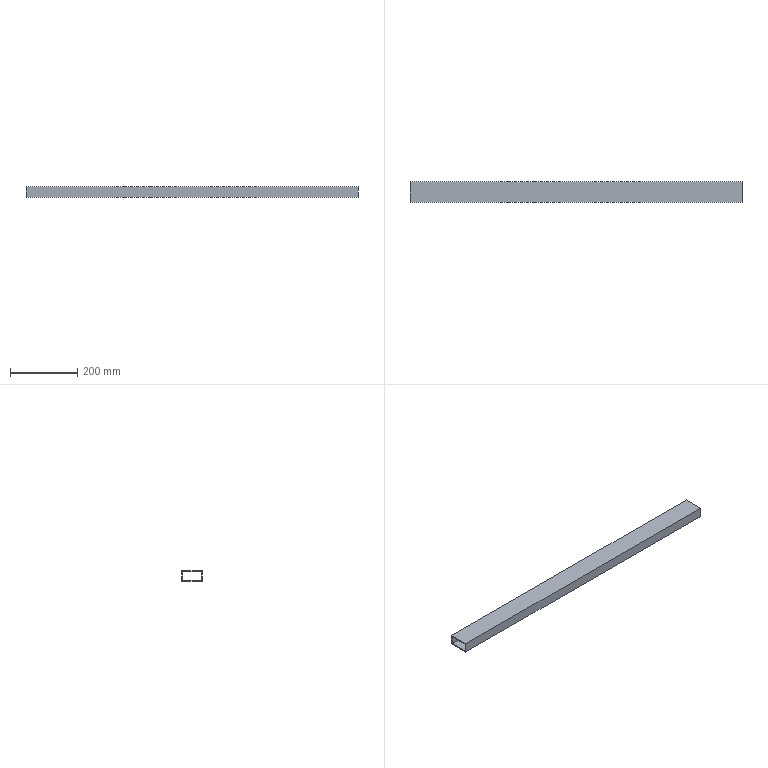Part | SolidWorks | features Cut 1, Extrusion 1 | 1 solid | 10 faces | box 986 x 60 x 30 mm | volume 496944 mm3 | plane 10
STEP:
#1=CARTESIAN_POINT('',(493.,-27.,27.));
#2=VERTEX_POINT('',#1);
#3=CARTESIAN_POINT('',(493.,27.,27.));
#4=VERTEX_POINT('',#3);
#5=CARTESIAN_POINT('',(493.,30.,27.));
#6=DIRECTION('',(0.,1.,0.));
#7=VECTOR('',#6,1000.);
#8=LINE('',#5,#7);
#9=EDGE_CURVE('',#2,#4,#8,.T.);
#10=ORIENTED_EDGE('',*,*,#9,.T.);
#11=CARTESIAN_POINT('',(493.,27.,3.));
#12=VERTEX_POINT('',#11);
#13=CARTESIAN_POINT('',(493.,27.,30.));
#14=DIRECTION('',(0.,0.,-1.));
#15=VECTOR('',#14,1000.);
#16=LINE('',#13,#15);
#17=EDGE_CURVE('',#4,#12,#16,.T.);
#18=ORIENTED_EDGE('',*,*,#17,.T.);
#19=CARTESIAN_POINT('',(493.,-27.,3.));
#20=VERTEX_POINT('',#19);
#21=CARTESIAN_POINT('',(493.,30.,3.));
#22=DIRECTION('',(0.,-1.,0.));
#23=VECTOR('',#22,1000.);
#24=LINE('',#21,#23);
#25=EDGE_CURVE('',#12,#20,#24,.T.);
#26=ORIENTED_EDGE('',*,*,#25,.T.);
#27=CARTESIAN_POINT('',(493.,-27.,30.));
#28=DIRECTION('',(0.,0.,1.));
#29=VECTOR('',#28,1000.);
#30=LINE('',#27,#29);
#31=EDGE_CURVE('',#20,#2,#30,.T.);
#32=ORIENTED_EDGE('',*,*,#31,.T.);
#33=EDGE_LOOP('',(#10,#18,#26,#32));
#34=FACE_BOUND('',#33,.T.);
#35=CARTESIAN_POINT('',(493.,-30.,0.));
#36=VERTEX_POINT('',#35);
#37=CARTESIAN_POINT('',(493.,30.,0.));
#38=VERTEX_POINT('',#37);
#39=CARTESIAN_POINT('',(493.,30.,0.));
#40=DIRECTION('',(0.,1.,0.));
#41=VECTOR('',#40,1000.);
#42=LINE('',#39,#41);
#43=EDGE_CURVE('',#36,#38,#42,.T.);
#44=ORIENTED_EDGE('',*,*,#43,.T.);
#45=CARTESIAN_POINT('',(493.,30.,30.));
#46=VERTEX_POINT('',#45);
#47=CARTESIAN_POINT('',(493.,30.,30.));
#48=DIRECTION('',(0.,0.,-1.));
#49=VECTOR('',#48,1000.);
#50=LINE('',#47,#49);
#51=EDGE_CURVE('',#46,#38,#50,.T.);
#52=ORIENTED_EDGE('',*,*,#51,.F.);
#53=CARTESIAN_POINT('',(493.,-30.,30.));
#54=VERTEX_POINT('',#53);
#55=CARTESIAN_POINT('',(493.,30.,30.));
#56=DIRECTION('',(0.,1.,0.));
#57=VECTOR('',#56,1000.);
#58=LINE('',#55,#57);
#59=EDGE_CURVE('',#54,#46,#58,.T.);
#60=ORIENTED_EDGE('',*,*,#59,.F.);
#61=CARTESIAN_POINT('',(493.,-30.,30.));
#62=DIRECTION('',(0.,0.,-1.));
#63=VECTOR('',#62,1000.);
#64=LINE('',#61,#63);
#65=EDGE_CURVE('',#54,#36,#64,.T.);
#66=ORIENTED_EDGE('',*,*,#65,.T.);
#67=EDGE_LOOP('',(#44,#52,#60,#66));
#68=FACE_OUTER_BOUND('',#67,.T.);
#69=CARTESIAN_POINT('',(493.,30.,30.));
#70=DIRECTION('',(-1.,0.,0.));
#71=DIRECTION('',(0.,0.,1.));
#72=AXIS2_PLACEMENT_3D('',#69,#70,#71);
#73=PLANE('',#72);
#74=ADVANCED_FACE('',(#34,#68),#73,.F.);
#75=CARTESIAN_POINT('',(-493.,30.,0.));
#76=VERTEX_POINT('',#75);
#77=CARTESIAN_POINT('',(-493.,30.,0.));
#78=DIRECTION('',(-1.,0.,0.));
#79=VECTOR('',#78,1000.);
#80=LINE('',#77,#79);
#81=EDGE_CURVE('',#38,#76,#80,.T.);
#82=ORIENTED_EDGE('',*,*,#81,.T.);
#83=CARTESIAN_POINT('',(-493.,30.,30.));
#84=VERTEX_POINT('',#83);
#85=CARTESIAN_POINT('',(-493.,30.,30.));
#86=DIRECTION('',(0.,0.,-1.));
#87=VECTOR('',#86,1000.);
#88=LINE('',#85,#87);
#89=EDGE_CURVE('',#84,#76,#88,.T.);
#90=ORIENTED_EDGE('',*,*,#89,.F.);
#91=CARTESIAN_POINT('',(-493.,30.,30.));
#92=DIRECTION('',(-1.,0.,0.));
#93=VECTOR('',#92,1000.);
#94=LINE('',#91,#93);
#95=EDGE_CURVE('',#46,#84,#94,.T.);
#96=ORIENTED_EDGE('',*,*,#95,.F.);
#97=ORIENTED_EDGE('',*,*,#51,.T.);
#98=EDGE_LOOP('',(#82,#90,#96,#97));
#99=FACE_OUTER_BOUND('',#98,.T.);
#100=CARTESIAN_POINT('',(-493.,30.,30.));
#101=DIRECTION('',(0.,-1.,0.));
#102=DIRECTION('',(0.,0.,-1.));
#103=AXIS2_PLACEMENT_3D('',#100,#101,#102);
#104=PLANE('',#103);
#105=ADVANCED_FACE('',(#99),#104,.F.);
#106=CARTESIAN_POINT('',(-493.,27.,3.));
#107=VERTEX_POINT('',#106);
#108=CARTESIAN_POINT('',(-493.,-27.,3.));
#109=VERTEX_POINT('',#108);
#110=CARTESIAN_POINT('',(-493.,27.,3.));
#111=DIRECTION('',(0.,-1.,0.));
#112=VECTOR('',#111,1000.);
#113=LINE('',#110,#112);
#114=EDGE_CURVE('',#107,#109,#113,.T.);
#115=ORIENTED_EDGE('',*,*,#114,.F.);
#116=CARTESIAN_POINT('',(-493.,27.,27.));
#117=VERTEX_POINT('',#116);
#118=CARTESIAN_POINT('',(-493.,27.,27.));
#119=DIRECTION('',(0.,0.,-1.));
#120=VECTOR('',#119,1000.);
#121=LINE('',#118,#120);
#122=EDGE_CURVE('',#117,#107,#121,.T.);
#123=ORIENTED_EDGE('',*,*,#122,.F.);
#124=CARTESIAN_POINT('',(-493.,-27.,27.));
#125=VERTEX_POINT('',#124);
#126=CARTESIAN_POINT('',(-493.,-27.,27.));
#127=DIRECTION('',(0.,1.,0.));
#128=VECTOR('',#127,1000.);
#129=LINE('',#126,#128);
#130=EDGE_CURVE('',#125,#117,#129,.T.);
#131=ORIENTED_EDGE('',*,*,#130,.F.);
#132=CARTESIAN_POINT('',(-493.,-27.,3.));
#133=DIRECTION('',(0.,0.,1.));
#134=VECTOR('',#133,1000.);
#135=LINE('',#132,#134);
#136=EDGE_CURVE('',#109,#125,#135,.T.);
#137=ORIENTED_EDGE('',*,*,#136,.F.);
#138=EDGE_LOOP('',(#115,#123,#131,#137));
#139=FACE_BOUND('',#138,.T.);
#140=CARTESIAN_POINT('',(-493.,-30.,0.));
#141=VERTEX_POINT('',#140);
#142=CARTESIAN_POINT('',(-493.,30.,0.));
#143=DIRECTION('',(0.,-1.,0.));
#144=VECTOR('',#143,1000.);
#145=LINE('',#142,#144);
#146=EDGE_CURVE('',#76,#141,#145,.T.);
#147=ORIENTED_EDGE('',*,*,#146,.T.);
#148=CARTESIAN_POINT('',(-493.,-30.,30.));
#149=VERTEX_POINT('',#148);
#150=CARTESIAN_POINT('',(-493.,-30.,30.));
#151=DIRECTION('',(0.,0.,-1.));
#152=VECTOR('',#151,1000.);
#153=LINE('',#150,#152);
#154=EDGE_CURVE('',#149,#141,#153,.T.);
#155=ORIENTED_EDGE('',*,*,#154,.F.);
#156=CARTESIAN_POINT('',(-493.,30.,30.));
#157=DIRECTION('',(0.,-1.,0.));
#158=VECTOR('',#157,1000.);
#159=LINE('',#156,#158);
#160=EDGE_CURVE('',#84,#149,#159,.T.);
#161=ORIENTED_EDGE('',*,*,#160,.F.);
#162=ORIENTED_EDGE('',*,*,#89,.T.);
#163=EDGE_LOOP('',(#147,#155,#161,#162));
#164=FACE_OUTER_BOUND('',#163,.T.);
#165=CARTESIAN_POINT('',(-493.,30.,30.));
#166=DIRECTION('',(1.,0.,0.));
#167=DIRECTION('',(0.,0.,-1.));
#168=AXIS2_PLACEMENT_3D('',#165,#166,#167);
#169=PLANE('',#168);
#170=ADVANCED_FACE('',(#139,#164),#169,.F.);
#171=CARTESIAN_POINT('',(-493.,-30.,0.));
#172=DIRECTION('',(1.,0.,0.));
#173=VECTOR('',#172,1000.);
#174=LINE('',#171,#173);
#175=EDGE_CURVE('',#141,#36,#174,.T.);
#176=ORIENTED_EDGE('',*,*,#175,.T.);
#177=ORIENTED_EDGE('',*,*,#65,.F.);
#178=CARTESIAN_POINT('',(-493.,-30.,30.));
#179=DIRECTION('',(1.,0.,0.));
#180=VECTOR('',#179,1000.);
#181=LINE('',#178,#180);
#182=EDGE_CURVE('',#149,#54,#181,.T.);
#183=ORIENTED_EDGE('',*,*,#182,.F.);
#184=ORIENTED_EDGE('',*,*,#154,.T.);
#185=EDGE_LOOP('',(#176,#177,#183,#184));
#186=FACE_OUTER_BOUND('',#185,.T.);
#187=CARTESIAN_POINT('',(-493.,-30.,30.));
#188=DIRECTION('',(0.,1.,0.));
#189=DIRECTION('',(0.,0.,1.));
#190=AXIS2_PLACEMENT_3D('',#187,#188,#189);
#191=PLANE('',#190);
#192=ADVANCED_FACE('',(#186),#191,.F.);
#193=ORIENTED_EDGE('',*,*,#59,.T.);
#194=ORIENTED_EDGE('',*,*,#95,.T.);
#195=ORIENTED_EDGE('',*,*,#160,.T.);
#196=ORIENTED_EDGE('',*,*,#182,.T.);
#197=EDGE_LOOP('',(#193,#194,#195,#196));
#198=FACE_OUTER_BOUND('',#197,.T.);
#199=CARTESIAN_POINT('',(0.,0.,30.));
#200=DIRECTION('',(0.,0.,1.));
#201=DIRECTION('',(1.,0.,0.));
#202=AXIS2_PLACEMENT_3D('',#199,#200,#201);
#203=PLANE('',#202);
#204=ADVANCED_FACE('',(#198),#203,.T.);
#205=ORIENTED_EDGE('',*,*,#43,.F.);
#206=ORIENTED_EDGE('',*,*,#175,.F.);
#207=ORIENTED_EDGE('',*,*,#146,.F.);
#208=ORIENTED_EDGE('',*,*,#81,.F.);
#209=EDGE_LOOP('',(#205,#206,#207,#208));
#210=FACE_OUTER_BOUND('',#209,.T.);
#211=CARTESIAN_POINT('',(0.,0.,0.));
#212=DIRECTION('',(0.,0.,1.));
#213=DIRECTION('',(1.,0.,0.));
#214=AXIS2_PLACEMENT_3D('',#211,#212,#213);
#215=PLANE('',#214);
#216=ADVANCED_FACE('',(#210),#215,.F.);
#217=CARTESIAN_POINT('',(1550.,27.,27.));
#218=DIRECTION('',(-1.,0.,0.));
#219=VECTOR('',#218,1000.);
#220=LINE('',#217,#219);
#221=EDGE_CURVE('',#4,#117,#220,.T.);
#222=ORIENTED_EDGE('',*,*,#221,.T.);
#223=ORIENTED_EDGE('',*,*,#122,.T.);
#224=CARTESIAN_POINT('',(1550.,27.,3.));
#225=DIRECTION('',(-1.,0.,0.));
#226=VECTOR('',#225,1000.);
#227=LINE('',#224,#226);
#228=EDGE_CURVE('',#12,#107,#227,.T.);
#229=ORIENTED_EDGE('',*,*,#228,.F.);
#230=ORIENTED_EDGE('',*,*,#17,.F.);
#231=EDGE_LOOP('',(#222,#223,#229,#230));
#232=FACE_OUTER_BOUND('',#231,.T.);
#233=CARTESIAN_POINT('',(1550.,27.,27.));
#234=DIRECTION('',(0.,1.,0.));
#235=DIRECTION('',(0.,0.,1.));
#236=AXIS2_PLACEMENT_3D('',#233,#234,#235);
#237=PLANE('',#236);
#238=ADVANCED_FACE('',(#232),#237,.F.);
#239=CARTESIAN_POINT('',(1550.,-27.,27.));
#240=DIRECTION('',(-1.,0.,0.));
#241=VECTOR('',#240,1000.);
#242=LINE('',#239,#241);
#243=EDGE_CURVE('',#2,#125,#242,.T.);
#244=ORIENTED_EDGE('',*,*,#243,.T.);
#245=ORIENTED_EDGE('',*,*,#130,.T.);
#246=ORIENTED_EDGE('',*,*,#221,.F.);
#247=ORIENTED_EDGE('',*,*,#9,.F.);
#248=EDGE_LOOP('',(#244,#245,#246,#247));
#249=FACE_OUTER_BOUND('',#248,.T.);
#250=CARTESIAN_POINT('',(1550.,-27.,27.));
#251=DIRECTION('',(0.,0.,1.));
#252=DIRECTION('',(1.,0.,0.));
#253=AXIS2_PLACEMENT_3D('',#250,#251,#252);
#254=PLANE('',#253);
#255=ADVANCED_FACE('',(#249),#254,.F.);
#256=CARTESIAN_POINT('',(1550.,-27.,3.));
#257=DIRECTION('',(-1.,0.,0.));
#258=VECTOR('',#257,1000.);
#259=LINE('',#256,#258);
#260=EDGE_CURVE('',#20,#109,#259,.T.);
#261=ORIENTED_EDGE('',*,*,#260,.T.);
#262=ORIENTED_EDGE('',*,*,#136,.T.);
#263=ORIENTED_EDGE('',*,*,#243,.F.);
#264=ORIENTED_EDGE('',*,*,#31,.F.);
#265=EDGE_LOOP('',(#261,#262,#263,#264));
#266=FACE_OUTER_BOUND('',#265,.T.);
#267=CARTESIAN_POINT('',(1550.,-27.,3.));
#268=DIRECTION('',(0.,-1.,0.));
#269=DIRECTION('',(0.,0.,-1.));
#270=AXIS2_PLACEMENT_3D('',#267,#268,#269);
#271=PLANE('',#270);
#272=ADVANCED_FACE('',(#266),#271,.F.);
#273=ORIENTED_EDGE('',*,*,#228,.T.);
#274=ORIENTED_EDGE('',*,*,#114,.T.);
#275=ORIENTED_EDGE('',*,*,#260,.F.);
#276=ORIENTED_EDGE('',*,*,#25,.F.);
#277=EDGE_LOOP('',(#273,#274,#275,#276));
#278=FACE_OUTER_BOUND('',#277,.T.);
#279=CARTESIAN_POINT('',(1550.,27.,3.));
#280=DIRECTION('',(0.,0.,-1.));
#281=DIRECTION('',(-1.,0.,0.));
#282=AXIS2_PLACEMENT_3D('',#279,#280,#281);
#283=PLANE('',#282);
#284=ADVANCED_FACE('',(#278),#283,.F.);
#285=CLOSED_SHELL('',(#74,#105,#170,#192,#204,#216,#238,#255,#272,#284));
#286=MANIFOLD_SOLID_BREP('',#285);
#287=CARTESIAN_POINT('',(0.,0.,0.));
#288=DIRECTION('',(0.,0.,1.));
#289=DIRECTION('',(1.,0.,0.));
#290=AXIS2_PLACEMENT_3D('',#287,#288,#289);
#291=(LENGTH_UNIT()NAMED_UNIT(*)SI_UNIT(.MILLI.,.METRE.));
#292=UNCERTAINTY_MEASURE_WITH_UNIT(LENGTH_MEASURE(0.00001),#291,'','');
#293=(NAMED_UNIT(*)PLANE_ANGLE_UNIT()SI_UNIT($,.RADIAN.));
#294=(NAMED_UNIT(*)SI_UNIT($,.STERADIAN.)SOLID_ANGLE_UNIT());
#295=(GEOMETRIC_REPRESENTATION_CONTEXT(3)GLOBAL_UNCERTAINTY_ASSIGNED_CONTEXT((#292))GLOBAL_UNIT_ASSIGNED_CONTEXT((#291,#293,#294))REPRESENTATION_CONTEXT('',''));
#296=ADVANCED_BREP_SHAPE_REPRESENTATION('',(#286,#290),#295);